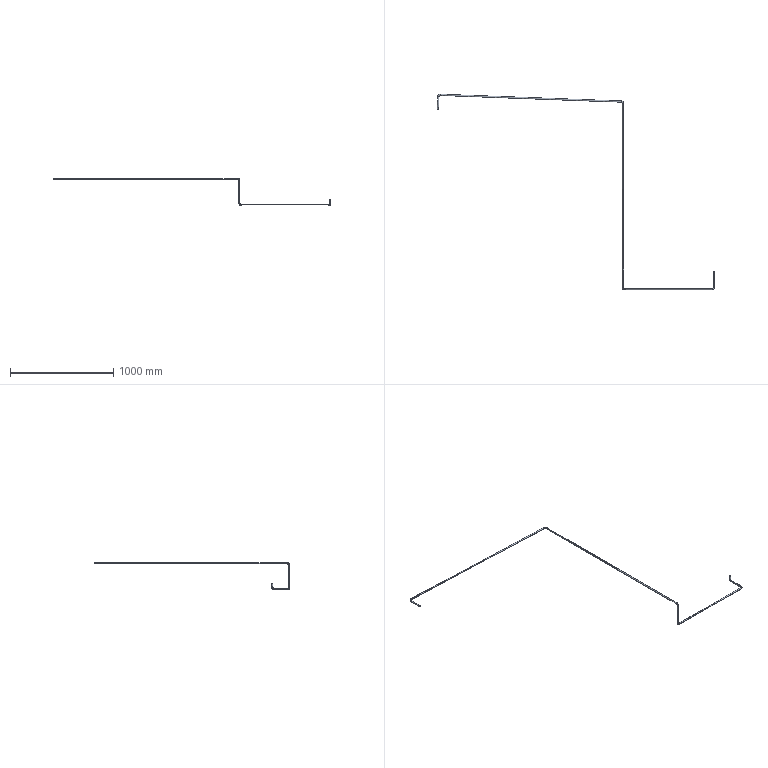Part | SolidWorks | features 3DProfileFeature 2, Sweep 1 | 1 solid | 54 faces | box 2689 x 1893 x 257.91 mm | volume 174349 mm3 | cylinder 28 | torus 24 | plane 2 | commonest cylinder face diameters 10 x14 12 x14